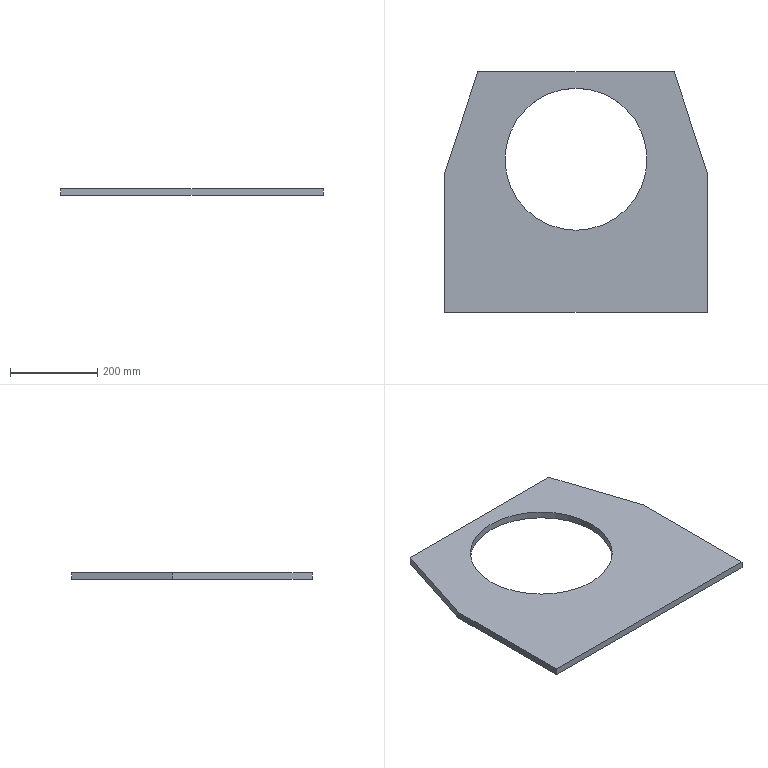Part | SolidWorks | features Extrusion 1 | 1 solid | 10 faces | box 600 x 550 x 16 mm | volume 3676677 mm3 | plane 8 | cylinder 2 | commonest cylinder face diameters 325 x2
STEP:
#1=CARTESIAN_POINT('',(-162.5,350.,8.));
#2=VERTEX_POINT('',#1);
#3=CARTESIAN_POINT('',(162.5,350.,8.));
#4=VERTEX_POINT('',#3);
#5=CARTESIAN_POINT('',(0.,350.,8.));
#6=DIRECTION('',(0.,0.,1.));
#7=DIRECTION('',(1.,0.,0.));
#8=AXIS2_PLACEMENT_3D('',#5,#6,#7);
#9=CIRCLE('',#8,162.5);
#10=EDGE_CURVE('',#2,#4,#9,.T.);
#11=ORIENTED_EDGE('',*,*,#10,.T.);
#12=CARTESIAN_POINT('',(162.5,350.,-8.));
#13=VERTEX_POINT('',#12);
#14=CARTESIAN_POINT('',(162.5,350.,8.));
#15=DIRECTION('',(0.,0.,-1.));
#16=VECTOR('',#15,1000.);
#17=LINE('',#14,#16);
#18=EDGE_CURVE('',#4,#13,#17,.T.);
#19=ORIENTED_EDGE('',*,*,#18,.T.);
#20=CARTESIAN_POINT('',(-162.5,350.,-8.));
#21=VERTEX_POINT('',#20);
#22=CARTESIAN_POINT('',(0.,350.,-8.));
#23=DIRECTION('',(0.,0.,1.));
#24=DIRECTION('',(1.,0.,0.));
#25=AXIS2_PLACEMENT_3D('',#22,#23,#24);
#26=CIRCLE('',#25,162.5);
#27=EDGE_CURVE('',#21,#13,#26,.T.);
#28=ORIENTED_EDGE('',*,*,#27,.F.);
#29=CARTESIAN_POINT('',(-162.5,350.,8.));
#30=DIRECTION('',(0.,0.,-1.));
#31=VECTOR('',#30,1000.);
#32=LINE('',#29,#31);
#33=EDGE_CURVE('',#2,#21,#32,.T.);
#34=ORIENTED_EDGE('',*,*,#33,.F.);
#35=EDGE_LOOP('',(#11,#19,#28,#34));
#36=FACE_OUTER_BOUND('',#35,.T.);
#37=CARTESIAN_POINT('',(0.,350.,8.));
#38=DIRECTION('',(0.,0.,-1.));
#39=DIRECTION('',(-1.,0.,0.));
#40=AXIS2_PLACEMENT_3D('',#37,#38,#39);
#41=CYLINDRICAL_SURFACE('',#40,162.5);
#42=ADVANCED_FACE('',(#36),#41,.F.);
#43=CARTESIAN_POINT('',(300.,320.,8.));
#44=VERTEX_POINT('',#43);
#45=CARTESIAN_POINT('',(225.,550.,8.));
#46=VERTEX_POINT('',#45);
#47=CARTESIAN_POINT('',(225.,550.,8.));
#48=DIRECTION('',(-0.31,0.9507,0.));
#49=VECTOR('',#48,1000.);
#50=LINE('',#47,#49);
#51=EDGE_CURVE('',#44,#46,#50,.T.);
#52=ORIENTED_EDGE('',*,*,#51,.T.);
#53=CARTESIAN_POINT('',(-225.,550.,8.));
#54=VERTEX_POINT('',#53);
#55=CARTESIAN_POINT('',(-225.,550.,8.));
#56=DIRECTION('',(-1.,0.,0.));
#57=VECTOR('',#56,1000.);
#58=LINE('',#55,#57);
#59=EDGE_CURVE('',#46,#54,#58,.T.);
#60=ORIENTED_EDGE('',*,*,#59,.T.);
#61=CARTESIAN_POINT('',(-300.,320.,8.));
#62=VERTEX_POINT('',#61);
#63=CARTESIAN_POINT('',(-225.,550.,8.));
#64=DIRECTION('',(-0.31,-0.9507,0.));
#65=VECTOR('',#64,1000.);
#66=LINE('',#63,#65);
#67=EDGE_CURVE('',#54,#62,#66,.T.);
#68=ORIENTED_EDGE('',*,*,#67,.T.);
#69=CARTESIAN_POINT('',(-300.,0.,8.));
#70=VERTEX_POINT('',#69);
#71=CARTESIAN_POINT('',(-300.,320.,8.));
#72=DIRECTION('',(0.,-1.,0.));
#73=VECTOR('',#72,1000.);
#74=LINE('',#71,#73);
#75=EDGE_CURVE('',#62,#70,#74,.T.);
#76=ORIENTED_EDGE('',*,*,#75,.T.);
#77=CARTESIAN_POINT('',(300.,0.,8.));
#78=VERTEX_POINT('',#77);
#79=CARTESIAN_POINT('',(300.,0.,8.));
#80=DIRECTION('',(1.,0.,0.));
#81=VECTOR('',#80,1000.);
#82=LINE('',#79,#81);
#83=EDGE_CURVE('',#70,#78,#82,.T.);
#84=ORIENTED_EDGE('',*,*,#83,.T.);
#85=CARTESIAN_POINT('',(300.,320.,8.));
#86=DIRECTION('',(0.,1.,0.));
#87=VECTOR('',#86,1000.);
#88=LINE('',#85,#87);
#89=EDGE_CURVE('',#78,#44,#88,.T.);
#90=ORIENTED_EDGE('',*,*,#89,.T.);
#91=EDGE_LOOP('',(#52,#60,#68,#76,#84,#90));
#92=FACE_OUTER_BOUND('',#91,.T.);
#93=ORIENTED_EDGE('',*,*,#10,.F.);
#94=CARTESIAN_POINT('',(0.,350.,8.));
#95=DIRECTION('',(0.,0.,1.));
#96=DIRECTION('',(1.,0.,0.));
#97=AXIS2_PLACEMENT_3D('',#94,#95,#96);
#98=CIRCLE('',#97,162.5);
#99=EDGE_CURVE('',#4,#2,#98,.T.);
#100=ORIENTED_EDGE('',*,*,#99,.F.);
#101=EDGE_LOOP('',(#93,#100));
#102=FACE_BOUND('',#101,.T.);
#103=CARTESIAN_POINT('',(0.,0.,8.));
#104=DIRECTION('',(0.,0.,-1.));
#105=DIRECTION('',(-1.,0.,0.));
#106=AXIS2_PLACEMENT_3D('',#103,#104,#105);
#107=PLANE('',#106);
#108=ADVANCED_FACE('',(#92,#102),#107,.F.);
#109=CARTESIAN_POINT('',(300.,320.,-8.));
#110=VERTEX_POINT('',#109);
#111=CARTESIAN_POINT('',(225.,550.,-8.));
#112=VERTEX_POINT('',#111);
#113=CARTESIAN_POINT('',(225.,550.,-8.));
#114=DIRECTION('',(-0.31,0.9507,0.));
#115=VECTOR('',#114,1000.);
#116=LINE('',#113,#115);
#117=EDGE_CURVE('',#110,#112,#116,.T.);
#118=ORIENTED_EDGE('',*,*,#117,.F.);
#119=CARTESIAN_POINT('',(300.,0.,-8.));
#120=VERTEX_POINT('',#119);
#121=CARTESIAN_POINT('',(300.,320.,-8.));
#122=DIRECTION('',(0.,1.,0.));
#123=VECTOR('',#122,1000.);
#124=LINE('',#121,#123);
#125=EDGE_CURVE('',#120,#110,#124,.T.);
#126=ORIENTED_EDGE('',*,*,#125,.F.);
#127=CARTESIAN_POINT('',(-300.,0.,-8.));
#128=VERTEX_POINT('',#127);
#129=CARTESIAN_POINT('',(300.,0.,-8.));
#130=DIRECTION('',(1.,0.,0.));
#131=VECTOR('',#130,1000.);
#132=LINE('',#129,#131);
#133=EDGE_CURVE('',#128,#120,#132,.T.);
#134=ORIENTED_EDGE('',*,*,#133,.F.);
#135=CARTESIAN_POINT('',(-300.,320.,-8.));
#136=VERTEX_POINT('',#135);
#137=CARTESIAN_POINT('',(-300.,320.,-8.));
#138=DIRECTION('',(0.,-1.,0.));
#139=VECTOR('',#138,1000.);
#140=LINE('',#137,#139);
#141=EDGE_CURVE('',#136,#128,#140,.T.);
#142=ORIENTED_EDGE('',*,*,#141,.F.);
#143=CARTESIAN_POINT('',(-225.,550.,-8.));
#144=VERTEX_POINT('',#143);
#145=CARTESIAN_POINT('',(-225.,550.,-8.));
#146=DIRECTION('',(-0.31,-0.9507,0.));
#147=VECTOR('',#146,1000.);
#148=LINE('',#145,#147);
#149=EDGE_CURVE('',#144,#136,#148,.T.);
#150=ORIENTED_EDGE('',*,*,#149,.F.);
#151=CARTESIAN_POINT('',(-225.,550.,-8.));
#152=DIRECTION('',(-1.,0.,0.));
#153=VECTOR('',#152,1000.);
#154=LINE('',#151,#153);
#155=EDGE_CURVE('',#112,#144,#154,.T.);
#156=ORIENTED_EDGE('',*,*,#155,.F.);
#157=EDGE_LOOP('',(#118,#126,#134,#142,#150,#156));
#158=FACE_OUTER_BOUND('',#157,.T.);
#159=ORIENTED_EDGE('',*,*,#27,.T.);
#160=CARTESIAN_POINT('',(0.,350.,-8.));
#161=DIRECTION('',(0.,0.,1.));
#162=DIRECTION('',(1.,0.,0.));
#163=AXIS2_PLACEMENT_3D('',#160,#161,#162);
#164=CIRCLE('',#163,162.5);
#165=EDGE_CURVE('',#13,#21,#164,.T.);
#166=ORIENTED_EDGE('',*,*,#165,.T.);
#167=EDGE_LOOP('',(#159,#166));
#168=FACE_BOUND('',#167,.T.);
#169=CARTESIAN_POINT('',(0.,0.,-8.));
#170=DIRECTION('',(0.,0.,-1.));
#171=DIRECTION('',(-1.,0.,0.));
#172=AXIS2_PLACEMENT_3D('',#169,#170,#171);
#173=PLANE('',#172);
#174=ADVANCED_FACE('',(#158,#168),#173,.T.);
#175=ORIENTED_EDGE('',*,*,#117,.T.);
#176=CARTESIAN_POINT('',(225.,550.,8.));
#177=DIRECTION('',(0.,0.,-1.));
#178=VECTOR('',#177,1000.);
#179=LINE('',#176,#178);
#180=EDGE_CURVE('',#46,#112,#179,.T.);
#181=ORIENTED_EDGE('',*,*,#180,.F.);
#182=ORIENTED_EDGE('',*,*,#51,.F.);
#183=CARTESIAN_POINT('',(300.,320.,8.));
#184=DIRECTION('',(0.,0.,-1.));
#185=VECTOR('',#184,1000.);
#186=LINE('',#183,#185);
#187=EDGE_CURVE('',#44,#110,#186,.T.);
#188=ORIENTED_EDGE('',*,*,#187,.T.);
#189=EDGE_LOOP('',(#175,#181,#182,#188));
#190=FACE_OUTER_BOUND('',#189,.T.);
#191=CARTESIAN_POINT('',(225.,550.,8.));
#192=DIRECTION('',(-0.9507,-0.31,0.));
#193=DIRECTION('',(0.31,-0.9507,0.));
#194=AXIS2_PLACEMENT_3D('',#191,#192,#193);
#195=PLANE('',#194);
#196=ADVANCED_FACE('',(#190),#195,.F.);
#197=ORIENTED_EDGE('',*,*,#155,.T.);
#198=CARTESIAN_POINT('',(-225.,550.,8.));
#199=DIRECTION('',(0.,0.,-1.));
#200=VECTOR('',#199,1000.);
#201=LINE('',#198,#200);
#202=EDGE_CURVE('',#54,#144,#201,.T.);
#203=ORIENTED_EDGE('',*,*,#202,.F.);
#204=ORIENTED_EDGE('',*,*,#59,.F.);
#205=ORIENTED_EDGE('',*,*,#180,.T.);
#206=EDGE_LOOP('',(#197,#203,#204,#205));
#207=FACE_OUTER_BOUND('',#206,.T.);
#208=CARTESIAN_POINT('',(-225.,550.,8.));
#209=DIRECTION('',(0.,-1.,0.));
#210=DIRECTION('',(0.,0.,-1.));
#211=AXIS2_PLACEMENT_3D('',#208,#209,#210);
#212=PLANE('',#211);
#213=ADVANCED_FACE('',(#207),#212,.F.);
#214=ORIENTED_EDGE('',*,*,#149,.T.);
#215=CARTESIAN_POINT('',(-300.,320.,8.));
#216=DIRECTION('',(0.,0.,-1.));
#217=VECTOR('',#216,1000.);
#218=LINE('',#215,#217);
#219=EDGE_CURVE('',#62,#136,#218,.T.);
#220=ORIENTED_EDGE('',*,*,#219,.F.);
#221=ORIENTED_EDGE('',*,*,#67,.F.);
#222=ORIENTED_EDGE('',*,*,#202,.T.);
#223=EDGE_LOOP('',(#214,#220,#221,#222));
#224=FACE_OUTER_BOUND('',#223,.T.);
#225=CARTESIAN_POINT('',(-225.,550.,8.));
#226=DIRECTION('',(0.9507,-0.31,0.));
#227=DIRECTION('',(0.31,0.9507,0.));
#228=AXIS2_PLACEMENT_3D('',#225,#226,#227);
#229=PLANE('',#228);
#230=ADVANCED_FACE('',(#224),#229,.F.);
#231=ORIENTED_EDGE('',*,*,#141,.T.);
#232=CARTESIAN_POINT('',(-300.,0.,8.));
#233=DIRECTION('',(0.,0.,-1.));
#234=VECTOR('',#233,1000.);
#235=LINE('',#232,#234);
#236=EDGE_CURVE('',#70,#128,#235,.T.);
#237=ORIENTED_EDGE('',*,*,#236,.F.);
#238=ORIENTED_EDGE('',*,*,#75,.F.);
#239=ORIENTED_EDGE('',*,*,#219,.T.);
#240=EDGE_LOOP('',(#231,#237,#238,#239));
#241=FACE_OUTER_BOUND('',#240,.T.);
#242=CARTESIAN_POINT('',(-300.,320.,8.));
#243=DIRECTION('',(1.,0.,0.));
#244=DIRECTION('',(0.,1.,0.));
#245=AXIS2_PLACEMENT_3D('',#242,#243,#244);
#246=PLANE('',#245);
#247=ADVANCED_FACE('',(#241),#246,.F.);
#248=ORIENTED_EDGE('',*,*,#133,.T.);
#249=CARTESIAN_POINT('',(300.,0.,8.));
#250=DIRECTION('',(0.,0.,-1.));
#251=VECTOR('',#250,1000.);
#252=LINE('',#249,#251);
#253=EDGE_CURVE('',#78,#120,#252,.T.);
#254=ORIENTED_EDGE('',*,*,#253,.F.);
#255=ORIENTED_EDGE('',*,*,#83,.F.);
#256=ORIENTED_EDGE('',*,*,#236,.T.);
#257=EDGE_LOOP('',(#248,#254,#255,#256));
#258=FACE_OUTER_BOUND('',#257,.T.);
#259=CARTESIAN_POINT('',(300.,0.,8.));
#260=DIRECTION('',(0.,1.,0.));
#261=DIRECTION('',(0.,0.,1.));
#262=AXIS2_PLACEMENT_3D('',#259,#260,#261);
#263=PLANE('',#262);
#264=ADVANCED_FACE('',(#258),#263,.F.);
#265=ORIENTED_EDGE('',*,*,#125,.T.);
#266=ORIENTED_EDGE('',*,*,#187,.F.);
#267=ORIENTED_EDGE('',*,*,#89,.F.);
#268=ORIENTED_EDGE('',*,*,#253,.T.);
#269=EDGE_LOOP('',(#265,#266,#267,#268));
#270=FACE_OUTER_BOUND('',#269,.T.);
#271=CARTESIAN_POINT('',(300.,320.,8.));
#272=DIRECTION('',(-1.,0.,0.));
#273=DIRECTION('',(0.,-1.,0.));
#274=AXIS2_PLACEMENT_3D('',#271,#272,#273);
#275=PLANE('',#274);
#276=ADVANCED_FACE('',(#270),#275,.F.);
#277=ORIENTED_EDGE('',*,*,#18,.F.);
#278=ORIENTED_EDGE('',*,*,#99,.T.);
#279=ORIENTED_EDGE('',*,*,#33,.T.);
#280=ORIENTED_EDGE('',*,*,#165,.F.);
#281=EDGE_LOOP('',(#277,#278,#279,#280));
#282=FACE_OUTER_BOUND('',#281,.T.);
#283=CARTESIAN_POINT('',(0.,350.,8.));
#284=DIRECTION('',(0.,0.,-1.));
#285=DIRECTION('',(-1.,0.,0.));
#286=AXIS2_PLACEMENT_3D('',#283,#284,#285);
#287=CYLINDRICAL_SURFACE('',#286,162.5);
#288=ADVANCED_FACE('',(#282),#287,.F.);
#289=CLOSED_SHELL('',(#42,#108,#174,#196,#213,#230,#247,#264,#276,#288));
#290=MANIFOLD_SOLID_BREP('',#289);
#291=CARTESIAN_POINT('',(0.,0.,0.));
#292=DIRECTION('',(0.,0.,1.));
#293=DIRECTION('',(1.,0.,0.));
#294=AXIS2_PLACEMENT_3D('',#291,#292,#293);
#295=(LENGTH_UNIT()NAMED_UNIT(*)SI_UNIT(.MILLI.,.METRE.));
#296=UNCERTAINTY_MEASURE_WITH_UNIT(LENGTH_MEASURE(0.00001),#295,'','');
#297=(NAMED_UNIT(*)PLANE_ANGLE_UNIT()SI_UNIT($,.RADIAN.));
#298=(NAMED_UNIT(*)SI_UNIT($,.STERADIAN.)SOLID_ANGLE_UNIT());
#299=(GEOMETRIC_REPRESENTATION_CONTEXT(3)GLOBAL_UNCERTAINTY_ASSIGNED_CONTEXT((#296))GLOBAL_UNIT_ASSIGNED_CONTEXT((#295,#297,#298))REPRESENTATION_CONTEXT('',''));
#300=ADVANCED_BREP_SHAPE_REPRESENTATION('',(#290,#294),#299);